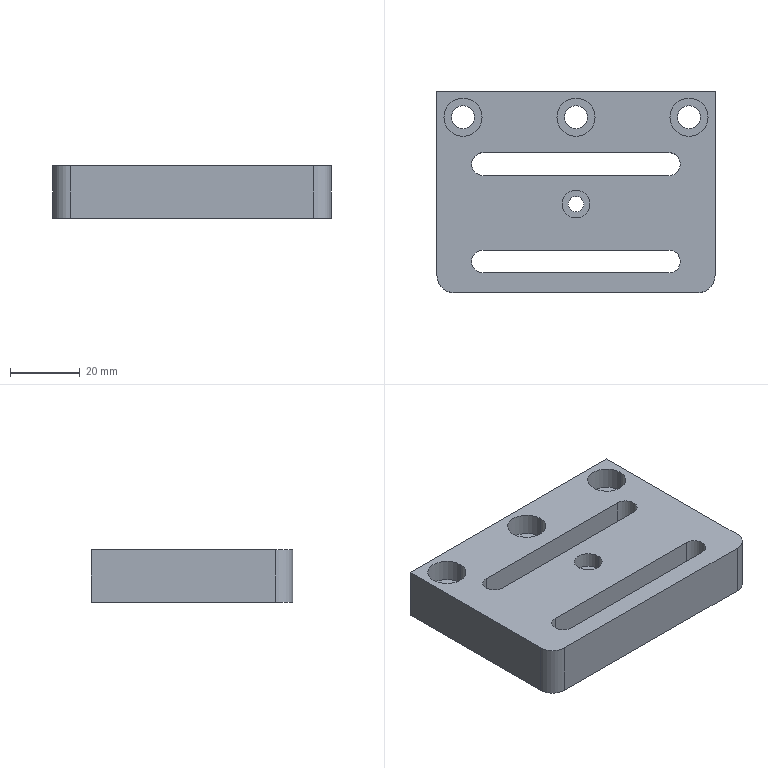Part | SolidWorks | features HoleWzd 3, Extrusion 1, Fillet 1 | 1 solid | 50 faces | box 80 x 58 x 15 mm | volume 50956 mm3 | cylinder 30 | plane 20 | commonest cylinder face diameters 6.6 x12 11 x12 4.5 x2 8 x2 10 x2
STEP:
#1=CARTESIAN_POINT('',(-38.,21.5,8.6));
#2=VERTEX_POINT('',#1);
#3=CARTESIAN_POINT('',(-27.,21.5,8.6));
#4=VERTEX_POINT('',#3);
#5=CARTESIAN_POINT('',(-32.5,21.5,8.6));
#6=DIRECTION('',(0.,0.,1.));
#7=DIRECTION('',(1.,0.,0.));
#8=AXIS2_PLACEMENT_3D('',#5,#6,#7);
#9=CIRCLE('',#8,5.5);
#10=EDGE_CURVE('',#2,#4,#9,.T.);
#11=ORIENTED_EDGE('',*,*,#10,.F.);
#12=CARTESIAN_POINT('',(-38.,21.5,15.));
#13=VERTEX_POINT('',#12);
#14=CARTESIAN_POINT('',(-38.,21.5,15.));
#15=DIRECTION('',(0.,0.,1.));
#16=VECTOR('',#15,1000.);
#17=LINE('',#14,#16);
#18=EDGE_CURVE('',#2,#13,#17,.T.);
#19=ORIENTED_EDGE('',*,*,#18,.T.);
#20=CARTESIAN_POINT('',(-27.,21.5,15.));
#21=VERTEX_POINT('',#20);
#22=CARTESIAN_POINT('',(-32.5,21.5,15.));
#23=DIRECTION('',(0.,0.,1.));
#24=DIRECTION('',(1.,0.,0.));
#25=AXIS2_PLACEMENT_3D('',#22,#23,#24);
#26=CIRCLE('',#25,5.5);
#27=EDGE_CURVE('',#13,#21,#26,.T.);
#28=ORIENTED_EDGE('',*,*,#27,.T.);
#29=CARTESIAN_POINT('',(-27.,21.5,15.));
#30=DIRECTION('',(0.,0.,1.));
#31=VECTOR('',#30,1000.);
#32=LINE('',#29,#31);
#33=EDGE_CURVE('',#4,#21,#32,.T.);
#34=ORIENTED_EDGE('',*,*,#33,.F.);
#35=EDGE_LOOP('',(#11,#19,#28,#34));
#36=FACE_OUTER_BOUND('',#35,.T.);
#37=CARTESIAN_POINT('',(-32.5,21.5,15.));
#38=DIRECTION('',(0.,0.,1.));
#39=DIRECTION('',(1.,0.,0.));
#40=AXIS2_PLACEMENT_3D('',#37,#38,#39);
#41=CYLINDRICAL_SURFACE('',#40,5.5);
#42=ADVANCED_FACE('',(#36),#41,.F.);
#43=CARTESIAN_POINT('',(-35.8,21.5,0.));
#44=VERTEX_POINT('',#43);
#45=CARTESIAN_POINT('',(-29.2,21.5,0.));
#46=VERTEX_POINT('',#45);
#47=CARTESIAN_POINT('',(-32.5,21.5,0.));
#48=DIRECTION('',(0.,0.,1.));
#49=DIRECTION('',(1.,0.,0.));
#50=AXIS2_PLACEMENT_3D('',#47,#48,#49);
#51=CIRCLE('',#50,3.3);
#52=EDGE_CURVE('',#44,#46,#51,.T.);
#53=ORIENTED_EDGE('',*,*,#52,.F.);
#54=CARTESIAN_POINT('',(-35.8,21.5,8.6));
#55=VERTEX_POINT('',#54);
#56=CARTESIAN_POINT('',(-35.8,21.5,15.));
#57=DIRECTION('',(0.,0.,1.));
#58=VECTOR('',#57,1000.);
#59=LINE('',#56,#58);
#60=EDGE_CURVE('',#44,#55,#59,.T.);
#61=ORIENTED_EDGE('',*,*,#60,.T.);
#62=CARTESIAN_POINT('',(-29.2,21.5,8.6));
#63=VERTEX_POINT('',#62);
#64=CARTESIAN_POINT('',(-32.5,21.5,8.6));
#65=DIRECTION('',(0.,0.,1.));
#66=DIRECTION('',(1.,0.,0.));
#67=AXIS2_PLACEMENT_3D('',#64,#65,#66);
#68=CIRCLE('',#67,3.3);
#69=EDGE_CURVE('',#55,#63,#68,.T.);
#70=ORIENTED_EDGE('',*,*,#69,.T.);
#71=CARTESIAN_POINT('',(-29.2,21.5,15.));
#72=DIRECTION('',(0.,0.,1.));
#73=VECTOR('',#72,1000.);
#74=LINE('',#71,#73);
#75=EDGE_CURVE('',#46,#63,#74,.T.);
#76=ORIENTED_EDGE('',*,*,#75,.F.);
#77=EDGE_LOOP('',(#53,#61,#70,#76));
#78=FACE_OUTER_BOUND('',#77,.T.);
#79=CARTESIAN_POINT('',(-32.5,21.5,15.));
#80=DIRECTION('',(0.,0.,1.));
#81=DIRECTION('',(1.,0.,0.));
#82=AXIS2_PLACEMENT_3D('',#79,#80,#81);
#83=CYLINDRICAL_SURFACE('',#82,3.3);
#84=ADVANCED_FACE('',(#78),#83,.F.);
#85=CARTESIAN_POINT('',(-5.5,21.5,8.6));
#86=VERTEX_POINT('',#85);
#87=CARTESIAN_POINT('',(5.5,21.5,8.6));
#88=VERTEX_POINT('',#87);
#89=CARTESIAN_POINT('',(0.,21.5,8.6));
#90=DIRECTION('',(0.,0.,1.));
#91=DIRECTION('',(1.,0.,0.));
#92=AXIS2_PLACEMENT_3D('',#89,#90,#91);
#93=CIRCLE('',#92,5.5);
#94=EDGE_CURVE('',#86,#88,#93,.T.);
#95=ORIENTED_EDGE('',*,*,#94,.F.);
#96=CARTESIAN_POINT('',(-5.5,21.5,15.));
#97=VERTEX_POINT('',#96);
#98=CARTESIAN_POINT('',(-5.5,21.5,15.));
#99=DIRECTION('',(0.,0.,1.));
#100=VECTOR('',#99,1000.);
#101=LINE('',#98,#100);
#102=EDGE_CURVE('',#86,#97,#101,.T.);
#103=ORIENTED_EDGE('',*,*,#102,.T.);
#104=CARTESIAN_POINT('',(5.5,21.5,15.));
#105=VERTEX_POINT('',#104);
#106=CARTESIAN_POINT('',(0.,21.5,15.));
#107=DIRECTION('',(0.,0.,1.));
#108=DIRECTION('',(1.,0.,0.));
#109=AXIS2_PLACEMENT_3D('',#106,#107,#108);
#110=CIRCLE('',#109,5.5);
#111=EDGE_CURVE('',#97,#105,#110,.T.);
#112=ORIENTED_EDGE('',*,*,#111,.T.);
#113=CARTESIAN_POINT('',(5.5,21.5,15.));
#114=DIRECTION('',(0.,0.,1.));
#115=VECTOR('',#114,1000.);
#116=LINE('',#113,#115);
#117=EDGE_CURVE('',#88,#105,#116,.T.);
#118=ORIENTED_EDGE('',*,*,#117,.F.);
#119=EDGE_LOOP('',(#95,#103,#112,#118));
#120=FACE_OUTER_BOUND('',#119,.T.);
#121=CARTESIAN_POINT('',(0.,21.5,15.));
#122=DIRECTION('',(0.,0.,1.));
#123=DIRECTION('',(1.,0.,0.));
#124=AXIS2_PLACEMENT_3D('',#121,#122,#123);
#125=CYLINDRICAL_SURFACE('',#124,5.5);
#126=ADVANCED_FACE('',(#120),#125,.F.);
#127=CARTESIAN_POINT('',(-3.3,21.5,0.));
#128=VERTEX_POINT('',#127);
#129=CARTESIAN_POINT('',(3.3,21.5,0.));
#130=VERTEX_POINT('',#129);
#131=CARTESIAN_POINT('',(0.,21.5,0.));
#132=DIRECTION('',(0.,0.,1.));
#133=DIRECTION('',(1.,0.,0.));
#134=AXIS2_PLACEMENT_3D('',#131,#132,#133);
#135=CIRCLE('',#134,3.3);
#136=EDGE_CURVE('',#128,#130,#135,.T.);
#137=ORIENTED_EDGE('',*,*,#136,.F.);
#138=CARTESIAN_POINT('',(-3.3,21.5,8.6));
#139=VERTEX_POINT('',#138);
#140=CARTESIAN_POINT('',(-3.3,21.5,15.));
#141=DIRECTION('',(0.,0.,1.));
#142=VECTOR('',#141,1000.);
#143=LINE('',#140,#142);
#144=EDGE_CURVE('',#128,#139,#143,.T.);
#145=ORIENTED_EDGE('',*,*,#144,.T.);
#146=CARTESIAN_POINT('',(3.3,21.5,8.6));
#147=VERTEX_POINT('',#146);
#148=CARTESIAN_POINT('',(0.,21.5,8.6));
#149=DIRECTION('',(0.,0.,1.));
#150=DIRECTION('',(1.,0.,0.));
#151=AXIS2_PLACEMENT_3D('',#148,#149,#150);
#152=CIRCLE('',#151,3.3);
#153=EDGE_CURVE('',#139,#147,#152,.T.);
#154=ORIENTED_EDGE('',*,*,#153,.T.);
#155=CARTESIAN_POINT('',(3.3,21.5,15.));
#156=DIRECTION('',(0.,0.,1.));
#157=VECTOR('',#156,1000.);
#158=LINE('',#155,#157);
#159=EDGE_CURVE('',#130,#147,#158,.T.);
#160=ORIENTED_EDGE('',*,*,#159,.F.);
#161=EDGE_LOOP('',(#137,#145,#154,#160));
#162=FACE_OUTER_BOUND('',#161,.T.);
#163=CARTESIAN_POINT('',(0.,21.5,15.));
#164=DIRECTION('',(0.,0.,1.));
#165=DIRECTION('',(1.,0.,0.));
#166=AXIS2_PLACEMENT_3D('',#163,#164,#165);
#167=CYLINDRICAL_SURFACE('',#166,3.3);
#168=ADVANCED_FACE('',(#162),#167,.F.);
#169=CARTESIAN_POINT('',(27.,21.5,8.6));
#170=VERTEX_POINT('',#169);
#171=CARTESIAN_POINT('',(38.,21.5,8.6));
#172=VERTEX_POINT('',#171);
#173=CARTESIAN_POINT('',(32.5,21.5,8.6));
#174=DIRECTION('',(0.,0.,1.));
#175=DIRECTION('',(1.,0.,0.));
#176=AXIS2_PLACEMENT_3D('',#173,#174,#175);
#177=CIRCLE('',#176,5.5);
#178=EDGE_CURVE('',#170,#172,#177,.T.);
#179=ORIENTED_EDGE('',*,*,#178,.F.);
#180=CARTESIAN_POINT('',(27.,21.5,15.));
#181=VERTEX_POINT('',#180);
#182=CARTESIAN_POINT('',(27.,21.5,15.));
#183=DIRECTION('',(0.,0.,1.));
#184=VECTOR('',#183,1000.);
#185=LINE('',#182,#184);
#186=EDGE_CURVE('',#170,#181,#185,.T.);
#187=ORIENTED_EDGE('',*,*,#186,.T.);
#188=CARTESIAN_POINT('',(38.,21.5,15.));
#189=VERTEX_POINT('',#188);
#190=CARTESIAN_POINT('',(32.5,21.5,15.));
#191=DIRECTION('',(0.,0.,1.));
#192=DIRECTION('',(1.,0.,0.));
#193=AXIS2_PLACEMENT_3D('',#190,#191,#192);
#194=CIRCLE('',#193,5.5);
#195=EDGE_CURVE('',#181,#189,#194,.T.);
#196=ORIENTED_EDGE('',*,*,#195,.T.);
#197=CARTESIAN_POINT('',(38.,21.5,15.));
#198=DIRECTION('',(0.,0.,1.));
#199=VECTOR('',#198,1000.);
#200=LINE('',#197,#199);
#201=EDGE_CURVE('',#172,#189,#200,.T.);
#202=ORIENTED_EDGE('',*,*,#201,.F.);
#203=EDGE_LOOP('',(#179,#187,#196,#202));
#204=FACE_OUTER_BOUND('',#203,.T.);
#205=CARTESIAN_POINT('',(32.5,21.5,15.));
#206=DIRECTION('',(0.,0.,1.));
#207=DIRECTION('',(1.,0.,0.));
#208=AXIS2_PLACEMENT_3D('',#205,#206,#207);
#209=CYLINDRICAL_SURFACE('',#208,5.5);
#210=ADVANCED_FACE('',(#204),#209,.F.);
#211=CARTESIAN_POINT('',(29.2,21.5,0.));
#212=VERTEX_POINT('',#211);
#213=CARTESIAN_POINT('',(35.8,21.5,0.));
#214=VERTEX_POINT('',#213);
#215=CARTESIAN_POINT('',(32.5,21.5,0.));
#216=DIRECTION('',(0.,0.,1.));
#217=DIRECTION('',(1.,0.,0.));
#218=AXIS2_PLACEMENT_3D('',#215,#216,#217);
#219=CIRCLE('',#218,3.3);
#220=EDGE_CURVE('',#212,#214,#219,.T.);
#221=ORIENTED_EDGE('',*,*,#220,.F.);
#222=CARTESIAN_POINT('',(29.2,21.5,8.6));
#223=VERTEX_POINT('',#222);
#224=CARTESIAN_POINT('',(29.2,21.5,15.));
#225=DIRECTION('',(0.,0.,1.));
#226=VECTOR('',#225,1000.);
#227=LINE('',#224,#226);
#228=EDGE_CURVE('',#212,#223,#227,.T.);
#229=ORIENTED_EDGE('',*,*,#228,.T.);
#230=CARTESIAN_POINT('',(35.8,21.5,8.6));
#231=VERTEX_POINT('',#230);
#232=CARTESIAN_POINT('',(32.5,21.5,8.6));
#233=DIRECTION('',(0.,0.,1.));
#234=DIRECTION('',(1.,0.,0.));
#235=AXIS2_PLACEMENT_3D('',#232,#233,#234);
#236=CIRCLE('',#235,3.3);
#237=EDGE_CURVE('',#223,#231,#236,.T.);
#238=ORIENTED_EDGE('',*,*,#237,.T.);
#239=CARTESIAN_POINT('',(35.8,21.5,15.));
#240=DIRECTION('',(0.,0.,1.));
#241=VECTOR('',#240,1000.);
#242=LINE('',#239,#241);
#243=EDGE_CURVE('',#214,#231,#242,.T.);
#244=ORIENTED_EDGE('',*,*,#243,.F.);
#245=EDGE_LOOP('',(#221,#229,#238,#244));
#246=FACE_OUTER_BOUND('',#245,.T.);
#247=CARTESIAN_POINT('',(32.5,21.5,15.));
#248=DIRECTION('',(0.,0.,1.));
#249=DIRECTION('',(1.,0.,0.));
#250=AXIS2_PLACEMENT_3D('',#247,#248,#249);
#251=CYLINDRICAL_SURFACE('',#250,3.3);
#252=ADVANCED_FACE('',(#246),#251,.F.);
#253=CARTESIAN_POINT('',(-4.,-3.5,10.6));
#254=VERTEX_POINT('',#253);
#255=CARTESIAN_POINT('',(4.,-3.5,10.6));
#256=VERTEX_POINT('',#255);
#257=CARTESIAN_POINT('',(0.,-3.5,10.6));
#258=DIRECTION('',(0.,0.,1.));
#259=DIRECTION('',(1.,0.,0.));
#260=AXIS2_PLACEMENT_3D('',#257,#258,#259);
#261=CIRCLE('',#260,4.);
#262=EDGE_CURVE('',#254,#256,#261,.T.);
#263=ORIENTED_EDGE('',*,*,#262,.F.);
#264=CARTESIAN_POINT('',(-4.,-3.5,15.));
#265=VERTEX_POINT('',#264);
#266=CARTESIAN_POINT('',(-4.,-3.5,15.));
#267=DIRECTION('',(0.,0.,1.));
#268=VECTOR('',#267,1000.);
#269=LINE('',#266,#268);
#270=EDGE_CURVE('',#254,#265,#269,.T.);
#271=ORIENTED_EDGE('',*,*,#270,.T.);
#272=CARTESIAN_POINT('',(4.,-3.5,15.));
#273=VERTEX_POINT('',#272);
#274=CARTESIAN_POINT('',(0.,-3.5,15.));
#275=DIRECTION('',(0.,0.,1.));
#276=DIRECTION('',(1.,0.,0.));
#277=AXIS2_PLACEMENT_3D('',#274,#275,#276);
#278=CIRCLE('',#277,4.);
#279=EDGE_CURVE('',#265,#273,#278,.T.);
#280=ORIENTED_EDGE('',*,*,#279,.T.);
#281=CARTESIAN_POINT('',(4.,-3.5,15.));
#282=DIRECTION('',(0.,0.,1.));
#283=VECTOR('',#282,1000.);
#284=LINE('',#281,#283);
#285=EDGE_CURVE('',#256,#273,#284,.T.);
#286=ORIENTED_EDGE('',*,*,#285,.F.);
#287=EDGE_LOOP('',(#263,#271,#280,#286));
#288=FACE_OUTER_BOUND('',#287,.T.);
#289=CARTESIAN_POINT('',(0.,-3.5,15.));
#290=DIRECTION('',(0.,0.,1.));
#291=DIRECTION('',(1.,0.,0.));
#292=AXIS2_PLACEMENT_3D('',#289,#290,#291);
#293=CYLINDRICAL_SURFACE('',#292,4.);
#294=ADVANCED_FACE('',(#288),#293,.F.);
#295=CARTESIAN_POINT('',(-2.25,-3.5,0.));
#296=VERTEX_POINT('',#295);
#297=CARTESIAN_POINT('',(2.25,-3.5,0.));
#298=VERTEX_POINT('',#297);
#299=CARTESIAN_POINT('',(0.,-3.5,0.));
#300=DIRECTION('',(0.,0.,1.));
#301=DIRECTION('',(1.,0.,0.));
#302=AXIS2_PLACEMENT_3D('',#299,#300,#301);
#303=CIRCLE('',#302,2.25);
#304=EDGE_CURVE('',#296,#298,#303,.T.);
#305=ORIENTED_EDGE('',*,*,#304,.F.);
#306=CARTESIAN_POINT('',(-2.25,-3.5,10.6));
#307=VERTEX_POINT('',#306);
#308=CARTESIAN_POINT('',(-2.25,-3.5,15.));
#309=DIRECTION('',(0.,0.,1.));
#310=VECTOR('',#309,1000.);
#311=LINE('',#308,#310);
#312=EDGE_CURVE('',#296,#307,#311,.T.);
#313=ORIENTED_EDGE('',*,*,#312,.T.);
#314=CARTESIAN_POINT('',(2.25,-3.5,10.6));
#315=VERTEX_POINT('',#314);
#316=CARTESIAN_POINT('',(0.,-3.5,10.6));
#317=DIRECTION('',(0.,0.,1.));
#318=DIRECTION('',(1.,0.,0.));
#319=AXIS2_PLACEMENT_3D('',#316,#317,#318);
#320=CIRCLE('',#319,2.25);
#321=EDGE_CURVE('',#307,#315,#320,.T.);
#322=ORIENTED_EDGE('',*,*,#321,.T.);
#323=CARTESIAN_POINT('',(2.25,-3.5,15.));
#324=DIRECTION('',(0.,0.,1.));
#325=VECTOR('',#324,1000.);
#326=LINE('',#323,#325);
#327=EDGE_CURVE('',#298,#315,#326,.T.);
#328=ORIENTED_EDGE('',*,*,#327,.F.);
#329=EDGE_LOOP('',(#305,#313,#322,#328));
#330=FACE_OUTER_BOUND('',#329,.T.);
#331=CARTESIAN_POINT('',(0.,-3.5,15.));
#332=DIRECTION('',(0.,0.,1.));
#333=DIRECTION('',(1.,0.,0.));
#334=AXIS2_PLACEMENT_3D('',#331,#332,#333);
#335=CYLINDRICAL_SURFACE('',#334,2.25);
#336=ADVANCED_FACE('',(#330),#335,.F.);
#337=CARTESIAN_POINT('',(-32.2,-20.,6.4));
#338=VERTEX_POINT('',#337);
#339=CARTESIAN_POINT('',(-26.7,-14.5,6.4));
#340=VERTEX_POINT('',#339);
#341=CARTESIAN_POINT('',(-26.7,-20.,6.4));
#342=DIRECTION('',(0.,0.,-1.));
#343=DIRECTION('',(-1.,0.,0.));
#344=AXIS2_PLACEMENT_3D('',#341,#342,#343);
#345=CIRCLE('',#344,5.5);
#346=EDGE_CURVE('',#338,#340,#345,.T.);
#347=ORIENTED_EDGE('',*,*,#346,.F.);
#348=CARTESIAN_POINT('',(-32.2,-20.,0.));
#349=VERTEX_POINT('',#348);
#350=CARTESIAN_POINT('',(-32.2,-20.,0.));
#351=DIRECTION('',(0.,0.,-1.));
#352=VECTOR('',#351,1000.);
#353=LINE('',#350,#352);
#354=EDGE_CURVE('',#338,#349,#353,.T.);
#355=ORIENTED_EDGE('',*,*,#354,.T.);
#356=CARTESIAN_POINT('',(-26.7,-14.5,0.));
#357=VERTEX_POINT('',#356);
#358=CARTESIAN_POINT('',(-26.7,-20.,0.));
#359=DIRECTION('',(0.,0.,-1.));
#360=DIRECTION('',(-1.,0.,0.));
#361=AXIS2_PLACEMENT_3D('',#358,#359,#360);
#362=CIRCLE('',#361,5.5);
#363=EDGE_CURVE('',#349,#357,#362,.T.);
#364=ORIENTED_EDGE('',*,*,#363,.T.);
#365=CARTESIAN_POINT('',(-26.7,-14.5,0.));
#366=DIRECTION('',(0.,0.,-1.));
#367=VECTOR('',#366,1000.);
#368=LINE('',#365,#367);
#369=EDGE_CURVE('',#340,#357,#368,.T.);
#370=ORIENTED_EDGE('',*,*,#369,.F.);
#371=EDGE_LOOP('',(#347,#355,#364,#370));
#372=FACE_OUTER_BOUND('',#371,.T.);
#373=CARTESIAN_POINT('',(-26.7,-20.,0.));
#374=DIRECTION('',(0.,0.,-1.));
#375=DIRECTION('',(-1.,0.,0.));
#376=AXIS2_PLACEMENT_3D('',#373,#374,#375);
#377=CYLINDRICAL_SURFACE('',#376,5.5);
#378=ADVANCED_FACE('',(#372),#377,.F.);
#379=CARTESIAN_POINT('',(-30.,-20.,15.));
#380=VERTEX_POINT('',#379);
#381=CARTESIAN_POINT('',(-26.7,-16.7,15.));
#382=VERTEX_POINT('',#381);
#383=CARTESIAN_POINT('',(-26.7,-20.,15.));
#384=DIRECTION('',(0.,0.,-1.));
#385=DIRECTION('',(-1.,0.,0.));
#386=AXIS2_PLACEMENT_3D('',#383,#384,#385);
#387=CIRCLE('',#386,3.3);
#388=EDGE_CURVE('',#380,#382,#387,.T.);
#389=ORIENTED_EDGE('',*,*,#388,.F.);
#390=CARTESIAN_POINT('',(-30.,-20.,6.4));
#391=VERTEX_POINT('',#390);
#392=CARTESIAN_POINT('',(-30.,-20.,0.));
#393=DIRECTION('',(0.,0.,-1.));
#394=VECTOR('',#393,1000.);
#395=LINE('',#392,#394);
#396=EDGE_CURVE('',#380,#391,#395,.T.);
#397=ORIENTED_EDGE('',*,*,#396,.T.);
#398=CARTESIAN_POINT('',(-26.7,-16.7,6.4));
#399=VERTEX_POINT('',#398);
#400=CARTESIAN_POINT('',(-26.7,-20.,6.4));
#401=DIRECTION('',(0.,0.,-1.));
#402=DIRECTION('',(-1.,0.,0.));
#403=AXIS2_PLACEMENT_3D('',#400,#401,#402);
#404=CIRCLE('',#403,3.3);
#405=EDGE_CURVE('',#391,#399,#404,.T.);
#406=ORIENTED_EDGE('',*,*,#405,.T.);
#407=CARTESIAN_POINT('',(-26.7,-16.7,0.));
#408=DIRECTION('',(0.,0.,-1.));
#409=VECTOR('',#408,1000.);
#410=LINE('',#407,#409);
#411=EDGE_CURVE('',#382,#399,#410,.T.);
#412=ORIENTED_EDGE('',*,*,#411,.F.);
#413=EDGE_LOOP('',(#389,#397,#406,#412));
#414=FACE_OUTER_BOUND('',#413,.T.);
#415=CARTESIAN_POINT('',(-26.7,-20.,0.));
#416=DIRECTION('',(0.,0.,-1.));
#417=DIRECTION('',(-1.,0.,0.));
#418=AXIS2_PLACEMENT_3D('',#415,#416,#417);
#419=CYLINDRICAL_SURFACE('',#418,3.3);
#420=ADVANCED_FACE('',(#414),#419,.F.);
#421=CARTESIAN_POINT('',(-32.2,8.,6.4));
#422=VERTEX_POINT('',#421);
#423=CARTESIAN_POINT('',(-26.7,13.5,6.4));
#424=VERTEX_POINT('',#423);
#425=CARTESIAN_POINT('',(-26.7,8.,6.4));
#426=DIRECTION('',(0.,0.,-1.));
#427=DIRECTION('',(-1.,0.,0.));
#428=AXIS2_PLACEMENT_3D('',#425,#426,#427);
#429=CIRCLE('',#428,5.5);
#430=EDGE_CURVE('',#422,#424,#429,.T.);
#431=ORIENTED_EDGE('',*,*,#430,.F.);
#432=CARTESIAN_POINT('',(-32.2,8.,0.));
#433=VERTEX_POINT('',#432);
#434=CARTESIAN_POINT('',(-32.2,8.,0.));
#435=DIRECTION('',(0.,0.,-1.));
#436=VECTOR('',#435,1000.);
#437=LINE('',#434,#436);
#438=EDGE_CURVE('',#422,#433,#437,.T.);
#439=ORIENTED_EDGE('',*,*,#438,.T.);
#440=CARTESIAN_POINT('',(-26.7,13.5,0.));
#441=VERTEX_POINT('',#440);
#442=CARTESIAN_POINT('',(-26.7,8.,0.));
#443=DIRECTION('',(0.,0.,-1.));
#444=DIRECTION('',(-1.,0.,0.));
#445=AXIS2_PLACEMENT_3D('',#442,#443,#444);
#446=CIRCLE('',#445,5.5);
#447=EDGE_CURVE('',#433,#441,#446,.T.);
#448=ORIENTED_EDGE('',*,*,#447,.T.);
#449=CARTESIAN_POINT('',(-26.7,13.5,0.));
#450=DIRECTION('',(0.,0.,-1.));
#451=VECTOR('',#450,1000.);
#452=LINE('',#449,#451);
#453=EDGE_CURVE('',#424,#441,#452,.T.);
#454=ORIENTED_EDGE('',*,*,#453,.F.);
#455=EDGE_LOOP('',(#431,#439,#448,#454));
#456=FACE_OUTER_BOUND('',#455,.T.);
#457=CARTESIAN_POINT('',(-26.7,8.,0.));
#458=DIRECTION('',(0.,0.,-1.));
#459=DIRECTION('',(-1.,0.,0.));
#460=AXIS2_PLACEMENT_3D('',#457,#458,#459);
#461=CYLINDRICAL_SURFACE('',#460,5.5);
#462=ADVANCED_FACE('',(#456),#461,.F.);
#463=CARTESIAN_POINT('',(-30.,8.,15.));
#464=VERTEX_POINT('',#463);
#465=CARTESIAN_POINT('',(-26.7,11.3,15.));
#466=VERTEX_POINT('',#465);
#467=CARTESIAN_POINT('',(-26.7,8.,15.));
#468=DIRECTION('',(0.,0.,-1.));
#469=DIRECTION('',(-1.,0.,0.));
#470=AXIS2_PLACEMENT_3D('',#467,#468,#469);
#471=CIRCLE('',#470,3.3);
#472=EDGE_CURVE('',#464,#466,#471,.T.);
#473=ORIENTED_EDGE('',*,*,#472,.F.);
#474=CARTESIAN_POINT('',(-30.,8.,6.4));
#475=VERTEX_POINT('',#474);
#476=CARTESIAN_POINT('',(-30.,8.,0.));
#477=DIRECTION('',(0.,0.,-1.));
#478=VECTOR('',#477,1000.);
#479=LINE('',#476,#478);
#480=EDGE_CURVE('',#464,#475,#479,.T.);
#481=ORIENTED_EDGE('',*,*,#480,.T.);
#482=CARTESIAN_POINT('',(-26.7,11.3,6.4));
#483=VERTEX_POINT('',#482);
#484=CARTESIAN_POINT('',(-26.7,8.,6.4));
#485=DIRECTION('',(0.,0.,-1.));
#486=DIRECTION('',(-1.,0.,0.));
#487=AXIS2_PLACEMENT_3D('',#484,#485,#486);
#488=CIRCLE('',#487,3.3);
#489=EDGE_CURVE('',#475,#483,#488,.T.);
#490=ORIENTED_EDGE('',*,*,#489,.T.);
#491=CARTESIAN_POINT('',(-26.7,11.3,0.));
#492=DIRECTION('',(0.,0.,-1.));
#493=VECTOR('',#492,1000.);
#494=LINE('',#491,#493);
#495=EDGE_CURVE('',#466,#483,#494,.T.);
#496=ORIENTED_EDGE('',*,*,#495,.F.);
#497=EDGE_LOOP('',(#473,#481,#490,#496));
#498=FACE_OUTER_BOUND('',#497,.T.);
#499=CARTESIAN_POINT('',(-26.7,8.,0.));
#500=DIRECTION('',(0.,0.,-1.));
#501=DIRECTION('',(-1.,0.,0.));
#502=AXIS2_PLACEMENT_3D('',#499,#500,#501);
#503=CYLINDRICAL_SURFACE('',#502,3.3);
#504=ADVANCED_FACE('',(#498),#503,.F.);
#505=CARTESIAN_POINT('',(40.,-24.,15.));
#506=VERTEX_POINT('',#505);
#507=CARTESIAN_POINT('',(40.,29.,15.));
#508=VERTEX_POINT('',#507);
#509=CARTESIAN_POINT('',(40.,29.,15.));
#510=DIRECTION('',(0.,1.,0.));
#511=VECTOR('',#510,1000.);
#512=LINE('',#509,#511);
#513=EDGE_CURVE('',#506,#508,#512,.T.);
#514=ORIENTED_EDGE('',*,*,#513,.F.);
#515=CARTESIAN_POINT('',(40.,-24.,0.));
#516=VERTEX_POINT('',#515);
#517=CARTESIAN_POINT('',(40.,-24.,15.));
#518=DIRECTION('',(0.,0.,-1.));
#519=VECTOR('',#518,1000.);
#520=LINE('',#517,#519);
#521=EDGE_CURVE('',#506,#516,#520,.T.);
#522=ORIENTED_EDGE('',*,*,#521,.T.);
#523=CARTESIAN_POINT('',(40.,29.,0.));
#524=VERTEX_POINT('',#523);
#525=CARTESIAN_POINT('',(40.,29.,0.));
#526=DIRECTION('',(0.,1.,0.));
#527=VECTOR('',#526,1000.);
#528=LINE('',#525,#527);
#529=EDGE_CURVE('',#516,#524,#528,.T.);
#530=ORIENTED_EDGE('',*,*,#529,.T.);
#531=CARTESIAN_POINT('',(40.,29.,15.));
#532=DIRECTION('',(0.,0.,-1.));
#533=VECTOR('',#532,1000.);
#534=LINE('',#531,#533);
#535=EDGE_CURVE('',#508,#524,#534,.T.);
#536=ORIENTED_EDGE('',*,*,#535,.F.);
#537=EDGE_LOOP('',(#514,#522,#530,#536));
#538=FACE_OUTER_BOUND('',#537,.T.);
#539=CARTESIAN_POINT('',(40.,29.,15.));
#540=DIRECTION('',(-1.,0.,0.));
#541=DIRECTION('',(0.,-1.,0.));
#542=AXIS2_PLACEMENT_3D('',#539,#540,#541);
#543=PLANE('',#542);
#544=ADVANCED_FACE('',(#538),#543,.F.);
#545=CARTESIAN_POINT('',(-40.,29.,0.));
#546=VERTEX_POINT('',#545);
#547=CARTESIAN_POINT('',(-40.,29.,0.));
#548=DIRECTION('',(-1.,0.,0.));
#549=VECTOR('',#548,1000.);
#550=LINE('',#547,#549);
#551=EDGE_CURVE('',#524,#546,#550,.T.);
#552=ORIENTED_EDGE('',*,*,#551,.T.);
#553=CARTESIAN_POINT('',(-40.,29.,15.));
#554=VERTEX_POINT('',#553);
#555=CARTESIAN_POINT('',(-40.,29.,15.));
#556=DIRECTION('',(0.,0.,-1.));
#557=VECTOR('',#556,1000.);
#558=LINE('',#555,#557);
#559=EDGE_CURVE('',#554,#546,#558,.T.);
#560=ORIENTED_EDGE('',*,*,#559,.F.);
#561=CARTESIAN_POINT('',(-40.,29.,15.));
#562=DIRECTION('',(-1.,0.,0.));
#563=VECTOR('',#562,1000.);
#564=LINE('',#561,#563);
#565=EDGE_CURVE('',#508,#554,#564,.T.);
#566=ORIENTED_EDGE('',*,*,#565,.F.);
#567=ORIENTED_EDGE('',*,*,#535,.T.);
#568=EDGE_LOOP('',(#552,#560,#566,#567));
#569=FACE_OUTER_BOUND('',#568,.T.);
#570=CARTESIAN_POINT('',(-40.,29.,15.));
#571=DIRECTION('',(0.,-1.,0.));
#572=DIRECTION('',(1.,0.,0.));
#573=AXIS2_PLACEMENT_3D('',#570,#571,#572);
#574=PLANE('',#573);
#575=ADVANCED_FACE('',(#569),#574,.F.);
#576=CARTESIAN_POINT('',(-40.,-24.,0.));
#577=VERTEX_POINT('',#576);
#578=CARTESIAN_POINT('',(-40.,29.,0.));
#579=DIRECTION('',(0.,-1.,0.));
#580=VECTOR('',#579,1000.);
#581=LINE('',#578,#580);
#582=EDGE_CURVE('',#546,#577,#581,.T.);
#583=ORIENTED_EDGE('',*,*,#582,.T.);
#584=CARTESIAN_POINT('',(-40.,-24.,15.));
#585=VERTEX_POINT('',#584);
#586=CARTESIAN_POINT('',(-40.,-24.,15.));
#587=DIRECTION('',(0.,0.,1.));
#588=VECTOR('',#587,1000.);
#589=LINE('',#586,#588);
#590=EDGE_CURVE('',#577,#585,#589,.T.);
#591=ORIENTED_EDGE('',*,*,#590,.T.);
#592=CARTESIAN_POINT('',(-40.,29.,15.));
#593=DIRECTION('',(0.,-1.,0.));
#594=VECTOR('',#593,1000.);
#595=LINE('',#592,#594);
#596=EDGE_CURVE('',#554,#585,#595,.T.);
#597=ORIENTED_EDGE('',*,*,#596,.F.);
#598=ORIENTED_EDGE('',*,*,#559,.T.);
#599=EDGE_LOOP('',(#583,#591,#597,#598));
#600=FACE_OUTER_BOUND('',#599,.T.);
#601=CARTESIAN_POINT('',(-40.,29.,15.));
#602=DIRECTION('',(1.,0.,0.));
#603=DIRECTION('',(0.,1.,0.));
#604=AXIS2_PLACEMENT_3D('',#601,#602,#603);
#605=PLANE('',#604);
#606=ADVANCED_FACE('',(#600),#605,.F.);
#607=CARTESIAN_POINT('',(-35.,-29.,0.));
#608=VERTEX_POINT('',#607);
#609=CARTESIAN_POINT('',(35.,-29.,0.));
#610=VERTEX_POINT('',#609);
#611=CARTESIAN_POINT('',(-40.,-29.,0.));
#612=DIRECTION('',(1.,0.,0.));
#613=VECTOR('',#612,1000.);
#614=LINE('',#611,#613);
#615=EDGE_CURVE('',#608,#610,#614,.T.);
#616=ORIENTED_EDGE('',*,*,#615,.T.);
#617=CARTESIAN_POINT('',(35.,-29.,15.));
#618=VERTEX_POINT('',#617);
#619=CARTESIAN_POINT('',(35.,-29.,15.));
#620=DIRECTION('',(0.,0.,1.));
#621=VECTOR('',#620,1000.);
#622=LINE('',#619,#621);
#623=EDGE_CURVE('',#610,#618,#622,.T.);
#624=ORIENTED_EDGE('',*,*,#623,.T.);
#625=CARTESIAN_POINT('',(-35.,-29.,15.));
#626=VERTEX_POINT('',#625);
#627=CARTESIAN_POINT('',(-40.,-29.,15.));
#628=DIRECTION('',(1.,0.,0.));
#629=VECTOR('',#628,1000.);
#630=LINE('',#627,#629);
#631=EDGE_CURVE('',#626,#618,#630,.T.);
#632=ORIENTED_EDGE('',*,*,#631,.F.);
#633=CARTESIAN_POINT('',(-35.,-29.,15.));
#634=DIRECTION('',(0.,0.,-1.));
#635=VECTOR('',#634,1000.);
#636=LINE('',#633,#635);
#637=EDGE_CURVE('',#626,#608,#636,.T.);
#638=ORIENTED_EDGE('',*,*,#637,.T.);
#639=EDGE_LOOP('',(#616,#624,#632,#638));
#640=FACE_OUTER_BOUND('',#639,.T.);
#641=CARTESIAN_POINT('',(-40.,-29.,15.));
#642=DIRECTION('',(0.,1.,0.));
#643=DIRECTION('',(0.,0.,1.));
#644=AXIS2_PLACEMENT_3D('',#641,#642,#643);
#645=PLANE('',#644);
#646=ADVANCED_FACE('',(#640),#645,.F.);
#647=CARTESIAN_POINT('',(-32.5,21.5,15.));
#648=DIRECTION('',(0.,0.,1.));
#649=DIRECTION('',(1.,0.,0.));
#650=AXIS2_PLACEMENT_3D('',#647,#648,#649);
#651=CIRCLE('',#650,5.5);
#652=EDGE_CURVE('',#21,#13,#651,.T.);
#653=ORIENTED_EDGE('',*,*,#652,.F.);
#654=ORIENTED_EDGE('',*,*,#27,.F.);
#655=EDGE_LOOP('',(#653,#654));
#656=FACE_BOUND('',#655,.T.);
#657=CARTESIAN_POINT('',(0.,21.5,15.));
#658=DIRECTION('',(0.,0.,1.));
#659=DIRECTION('',(1.,0.,0.));
#660=AXIS2_PLACEMENT_3D('',#657,#658,#659);
#661=CIRCLE('',#660,5.5);
#662=EDGE_CURVE('',#105,#97,#661,.T.);
#663=ORIENTED_EDGE('',*,*,#662,.F.);
#664=ORIENTED_EDGE('',*,*,#111,.F.);
#665=EDGE_LOOP('',(#663,#664));
#666=FACE_BOUND('',#665,.T.);
#667=CARTESIAN_POINT('',(32.5,21.5,15.));
#668=DIRECTION('',(0.,0.,1.));
#669=DIRECTION('',(1.,0.,0.));
#670=AXIS2_PLACEMENT_3D('',#667,#668,#669);
#671=CIRCLE('',#670,5.5);
#672=EDGE_CURVE('',#189,#181,#671,.T.);
#673=ORIENTED_EDGE('',*,*,#672,.F.);
#674=ORIENTED_EDGE('',*,*,#195,.F.);
#675=EDGE_LOOP('',(#673,#674));
#676=FACE_BOUND('',#675,.T.);
#677=CARTESIAN_POINT('',(0.,-3.5,15.));
#678=DIRECTION('',(0.,0.,1.));
#679=DIRECTION('',(1.,0.,0.));
#680=AXIS2_PLACEMENT_3D('',#677,#678,#679);
#681=CIRCLE('',#680,4.);
#682=EDGE_CURVE('',#273,#265,#681,.T.);
#683=ORIENTED_EDGE('',*,*,#682,.F.);
#684=ORIENTED_EDGE('',*,*,#279,.F.);
#685=EDGE_LOOP('',(#683,#684));
#686=FACE_BOUND('',#685,.T.);
#687=CARTESIAN_POINT('',(26.7,-16.7,15.));
#688=VERTEX_POINT('',#687);
#689=CARTESIAN_POINT('',(26.7,-23.3,15.));
#690=VERTEX_POINT('',#689);
#691=CARTESIAN_POINT('',(26.7,-20.,15.));
#692=DIRECTION('',(0.,0.,-1.));
#693=DIRECTION('',(-1.,0.,0.));
#694=AXIS2_PLACEMENT_3D('',#691,#692,#693);
#695=CIRCLE('',#694,3.3);
#696=EDGE_CURVE('',#688,#690,#695,.T.);
#697=ORIENTED_EDGE('',*,*,#696,.T.);
#698=CARTESIAN_POINT('',(-26.7,-23.3,15.));
#699=VERTEX_POINT('',#698);
#700=CARTESIAN_POINT('',(-26.7,-23.3,15.));
#701=DIRECTION('',(1.,0.,0.));
#702=VECTOR('',#701,1000.);
#703=LINE('',#700,#702);
#704=EDGE_CURVE('',#699,#690,#703,.T.);
#705=ORIENTED_EDGE('',*,*,#704,.F.);
#706=CARTESIAN_POINT('',(-26.7,-20.,15.));
#707=DIRECTION('',(0.,0.,-1.));
#708=DIRECTION('',(-1.,0.,0.));
#709=AXIS2_PLACEMENT_3D('',#706,#707,#708);
#710=CIRCLE('',#709,3.3);
#711=EDGE_CURVE('',#699,#380,#710,.T.);
#712=ORIENTED_EDGE('',*,*,#711,.T.);
#713=ORIENTED_EDGE('',*,*,#388,.T.);
#714=CARTESIAN_POINT('',(-26.7,-16.7,15.));
#715=DIRECTION('',(1.,0.,0.));
#716=VECTOR('',#715,1000.);
#717=LINE('',#714,#716);
#718=EDGE_CURVE('',#382,#688,#717,.T.);
#719=ORIENTED_EDGE('',*,*,#718,.T.);
#720=EDGE_LOOP('',(#697,#705,#712,#713,#719));
#721=FACE_BOUND('',#720,.T.);
#722=CARTESIAN_POINT('',(26.7,11.3,15.));
#723=VERTEX_POINT('',#722);
#724=CARTESIAN_POINT('',(26.7,4.7,15.));
#725=VERTEX_POINT('',#724);
#726=CARTESIAN_POINT('',(26.7,8.,15.));
#727=DIRECTION('',(0.,0.,-1.));
#728=DIRECTION('',(-1.,0.,0.));
#729=AXIS2_PLACEMENT_3D('',#726,#727,#728);
#730=CIRCLE('',#729,3.3);
#731=EDGE_CURVE('',#723,#725,#730,.T.);
#732=ORIENTED_EDGE('',*,*,#731,.T.);
#733=CARTESIAN_POINT('',(-26.7,4.7,15.));
#734=VERTEX_POINT('',#733);
#735=CARTESIAN_POINT('',(-26.7,4.7,15.));
#736=DIRECTION('',(1.,0.,0.));
#737=VECTOR('',#736,1000.);
#738=LINE('',#735,#737);
#739=EDGE_CURVE('',#734,#725,#738,.T.);
#740=ORIENTED_EDGE('',*,*,#739,.F.);
#741=CARTESIAN_POINT('',(-26.7,8.,15.));
#742=DIRECTION('',(0.,0.,-1.));
#743=DIRECTION('',(-1.,0.,0.));
#744=AXIS2_PLACEMENT_3D('',#741,#742,#743);
#745=CIRCLE('',#744,3.3);
#746=EDGE_CURVE('',#734,#464,#745,.T.);
#747=ORIENTED_EDGE('',*,*,#746,.T.);
#748=ORIENTED_EDGE('',*,*,#472,.T.);
#749=CARTESIAN_POINT('',(-26.7,11.3,15.));
#750=DIRECTION('',(1.,0.,0.));
#751=VECTOR('',#750,1000.);
#752=LINE('',#749,#751);
#753=EDGE_CURVE('',#466,#723,#752,.T.);
#754=ORIENTED_EDGE('',*,*,#753,.T.);
#755=EDGE_LOOP('',(#732,#740,#747,#748,#754));
#756=FACE_BOUND('',#755,.T.);
#757=ORIENTED_EDGE('',*,*,#631,.T.);
#758=CARTESIAN_POINT('',(35.,-24.,15.));
#759=DIRECTION('',(0.,0.,1.));
#760=DIRECTION('',(1.,0.,0.));
#761=AXIS2_PLACEMENT_3D('',#758,#759,#760);
#762=CIRCLE('',#761,5.);
#763=EDGE_CURVE('',#618,#506,#762,.T.);
#764=ORIENTED_EDGE('',*,*,#763,.T.);
#765=ORIENTED_EDGE('',*,*,#513,.T.);
#766=ORIENTED_EDGE('',*,*,#565,.T.);
#767=ORIENTED_EDGE('',*,*,#596,.T.);
#768=CARTESIAN_POINT('',(-35.,-24.,15.));
#769=DIRECTION('',(0.,0.,1.));
#770=DIRECTION('',(1.,0.,0.));
#771=AXIS2_PLACEMENT_3D('',#768,#769,#770);
#772=CIRCLE('',#771,5.);
#773=EDGE_CURVE('',#585,#626,#772,.T.);
#774=ORIENTED_EDGE('',*,*,#773,.T.);
#775=EDGE_LOOP('',(#757,#764,#765,#766,#767,#774));
#776=FACE_OUTER_BOUND('',#775,.T.);
#777=CARTESIAN_POINT('',(0.,0.,15.));
#778=DIRECTION('',(0.,0.,1.));
#779=DIRECTION('',(1.,0.,0.));
#780=AXIS2_PLACEMENT_3D('',#777,#778,#779);
#781=PLANE('',#780);
#782=ADVANCED_FACE('',(#656,#666,#676,#686,#721,#756,#776),#781,.T.);
#783=CARTESIAN_POINT('',(-32.5,21.5,0.));
#784=DIRECTION('',(0.,0.,1.));
#785=DIRECTION('',(1.,0.,0.));
#786=AXIS2_PLACEMENT_3D('',#783,#784,#785);
#787=CIRCLE('',#786,3.3);
#788=EDGE_CURVE('',#46,#44,#787,.T.);
#789=ORIENTED_EDGE('',*,*,#788,.T.);
#790=ORIENTED_EDGE('',*,*,#52,.T.);
#791=EDGE_LOOP('',(#789,#790));
#792=FACE_BOUND('',#791,.T.);
#793=CARTESIAN_POINT('',(0.,21.5,0.));
#794=DIRECTION('',(0.,0.,1.));
#795=DIRECTION('',(1.,0.,0.));
#796=AXIS2_PLACEMENT_3D('',#793,#794,#795);
#797=CIRCLE('',#796,3.3);
#798=EDGE_CURVE('',#130,#128,#797,.T.);
#799=ORIENTED_EDGE('',*,*,#798,.T.);
#800=ORIENTED_EDGE('',*,*,#136,.T.);
#801=EDGE_LOOP('',(#799,#800));
#802=FACE_BOUND('',#801,.T.);
#803=CARTESIAN_POINT('',(32.5,21.5,0.));
#804=DIRECTION('',(0.,0.,1.));
#805=DIRECTION('',(1.,0.,0.));
#806=AXIS2_PLACEMENT_3D('',#803,#804,#805);
#807=CIRCLE('',#806,3.3);
#808=EDGE_CURVE('',#214,#212,#807,.T.);
#809=ORIENTED_EDGE('',*,*,#808,.T.);
#810=ORIENTED_EDGE('',*,*,#220,.T.);
#811=EDGE_LOOP('',(#809,#810));
#812=FACE_BOUND('',#811,.T.);
#813=CARTESIAN_POINT('',(0.,-3.5,0.));
#814=DIRECTION('',(0.,0.,1.));
#815=DIRECTION('',(1.,0.,0.));
#816=AXIS2_PLACEMENT_3D('',#813,#814,#815);
#817=CIRCLE('',#816,2.25);
#818=EDGE_CURVE('',#298,#296,#817,.T.);
#819=ORIENTED_EDGE('',*,*,#818,.T.);
#820=ORIENTED_EDGE('',*,*,#304,.T.);
#821=EDGE_LOOP('',(#819,#820));
#822=FACE_BOUND('',#821,.T.);
#823=CARTESIAN_POINT('',(26.7,-14.5,0.));
#824=VERTEX_POINT('',#823);
#825=CARTESIAN_POINT('',(26.7,-25.5,0.));
#826=VERTEX_POINT('',#825);
#827=CARTESIAN_POINT('',(26.7,-20.,0.));
#828=DIRECTION('',(0.,0.,-1.));
#829=DIRECTION('',(-1.,0.,0.));
#830=AXIS2_PLACEMENT_3D('',#827,#828,#829);
#831=CIRCLE('',#830,5.5);
#832=EDGE_CURVE('',#824,#826,#831,.T.);
#833=ORIENTED_EDGE('',*,*,#832,.F.);
#834=CARTESIAN_POINT('',(-26.7,-14.5,0.));
#835=DIRECTION('',(1.,0.,0.));
#836=VECTOR('',#835,1000.);
#837=LINE('',#834,#836);
#838=EDGE_CURVE('',#357,#824,#837,.T.);
#839=ORIENTED_EDGE('',*,*,#838,.F.);
#840=ORIENTED_EDGE('',*,*,#363,.F.);
#841=CARTESIAN_POINT('',(-26.7,-25.5,0.));
#842=VERTEX_POINT('',#841);
#843=CARTESIAN_POINT('',(-26.7,-20.,0.));
#844=DIRECTION('',(0.,0.,-1.));
#845=DIRECTION('',(-1.,0.,0.));
#846=AXIS2_PLACEMENT_3D('',#843,#844,#845);
#847=CIRCLE('',#846,5.5);
#848=EDGE_CURVE('',#842,#349,#847,.T.);
#849=ORIENTED_EDGE('',*,*,#848,.F.);
#850=CARTESIAN_POINT('',(-26.7,-25.5,0.));
#851=DIRECTION('',(1.,0.,0.));
#852=VECTOR('',#851,1000.);
#853=LINE('',#850,#852);
#854=EDGE_CURVE('',#842,#826,#853,.T.);
#855=ORIENTED_EDGE('',*,*,#854,.T.);
#856=EDGE_LOOP('',(#833,#839,#840,#849,#855));
#857=FACE_BOUND('',#856,.T.);
#858=CARTESIAN_POINT('',(-26.7,2.5,0.));
#859=VERTEX_POINT('',#858);
#860=CARTESIAN_POINT('',(-26.7,8.,0.));
#861=DIRECTION('',(0.,0.,-1.));
#862=DIRECTION('',(-1.,0.,0.));
#863=AXIS2_PLACEMENT_3D('',#860,#861,#862);
#864=CIRCLE('',#863,5.5);
#865=EDGE_CURVE('',#859,#433,#864,.T.);
#866=ORIENTED_EDGE('',*,*,#865,.F.);
#867=CARTESIAN_POINT('',(26.7,2.5,0.));
#868=VERTEX_POINT('',#867);
#869=CARTESIAN_POINT('',(-26.7,2.5,0.));
#870=DIRECTION('',(1.,0.,0.));
#871=VECTOR('',#870,1000.);
#872=LINE('',#869,#871);
#873=EDGE_CURVE('',#859,#868,#872,.T.);
#874=ORIENTED_EDGE('',*,*,#873,.T.);
#875=CARTESIAN_POINT('',(26.7,13.5,0.));
#876=VERTEX_POINT('',#875);
#877=CARTESIAN_POINT('',(26.7,8.,0.));
#878=DIRECTION('',(0.,0.,-1.));
#879=DIRECTION('',(-1.,0.,0.));
#880=AXIS2_PLACEMENT_3D('',#877,#878,#879);
#881=CIRCLE('',#880,5.5);
#882=EDGE_CURVE('',#876,#868,#881,.T.);
#883=ORIENTED_EDGE('',*,*,#882,.F.);
#884=CARTESIAN_POINT('',(-26.7,13.5,0.));
#885=DIRECTION('',(1.,0.,0.));
#886=VECTOR('',#885,1000.);
#887=LINE('',#884,#886);
#888=EDGE_CURVE('',#441,#876,#887,.T.);
#889=ORIENTED_EDGE('',*,*,#888,.F.);
#890=ORIENTED_EDGE('',*,*,#447,.F.);
#891=EDGE_LOOP('',(#866,#874,#883,#889,#890));
#892=FACE_BOUND('',#891,.T.);
#893=ORIENTED_EDGE('',*,*,#529,.F.);
#894=CARTESIAN_POINT('',(35.,-24.,0.));
#895=DIRECTION('',(0.,0.,-1.));
#896=DIRECTION('',(1.,0.,0.));
#897=AXIS2_PLACEMENT_3D('',#894,#895,#896);
#898=CIRCLE('',#897,5.);
#899=EDGE_CURVE('',#516,#610,#898,.T.);
#900=ORIENTED_EDGE('',*,*,#899,.T.);
#901=ORIENTED_EDGE('',*,*,#615,.F.);
#902=CARTESIAN_POINT('',(-35.,-24.,0.));
#903=DIRECTION('',(0.,0.,-1.));
#904=DIRECTION('',(1.,0.,0.));
#905=AXIS2_PLACEMENT_3D('',#902,#903,#904);
#906=CIRCLE('',#905,5.);
#907=EDGE_CURVE('',#608,#577,#906,.T.);
#908=ORIENTED_EDGE('',*,*,#907,.T.);
#909=ORIENTED_EDGE('',*,*,#582,.F.);
#910=ORIENTED_EDGE('',*,*,#551,.F.);
#911=EDGE_LOOP('',(#893,#900,#901,#908,#909,#910));
#912=FACE_OUTER_BOUND('',#911,.T.);
#913=CARTESIAN_POINT('',(0.,0.,0.));
#914=DIRECTION('',(0.,0.,1.));
#915=DIRECTION('',(1.,0.,0.));
#916=AXIS2_PLACEMENT_3D('',#913,#914,#915);
#917=PLANE('',#916);
#918=ADVANCED_FACE('',(#792,#802,#812,#822,#857,#892,#912),#917,.F.);
#919=ORIENTED_EDGE('',*,*,#731,.F.);
#920=CARTESIAN_POINT('',(26.7,11.3,6.4));
#921=VERTEX_POINT('',#920);
#922=CARTESIAN_POINT('',(26.7,11.3,0.));
#923=DIRECTION('',(0.,0.,1.));
#924=VECTOR('',#923,1000.);
#925=LINE('',#922,#924);
#926=EDGE_CURVE('',#921,#723,#925,.T.);
#927=ORIENTED_EDGE('',*,*,#926,.F.);
#928=CARTESIAN_POINT('',(26.7,4.7,6.4));
#929=VERTEX_POINT('',#928);
#930=CARTESIAN_POINT('',(26.7,8.,6.4));
#931=DIRECTION('',(0.,0.,-1.));
#932=DIRECTION('',(-1.,0.,0.));
#933=AXIS2_PLACEMENT_3D('',#930,#931,#932);
#934=CIRCLE('',#933,3.3);
#935=EDGE_CURVE('',#921,#929,#934,.T.);
#936=ORIENTED_EDGE('',*,*,#935,.T.);
#937=CARTESIAN_POINT('',(26.7,4.7,0.));
#938=DIRECTION('',(0.,0.,-1.));
#939=VECTOR('',#938,1000.);
#940=LINE('',#937,#939);
#941=EDGE_CURVE('',#725,#929,#940,.T.);
#942=ORIENTED_EDGE('',*,*,#941,.F.);
#943=EDGE_LOOP('',(#919,#927,#936,#942));
#944=FACE_OUTER_BOUND('',#943,.T.);
#945=CARTESIAN_POINT('',(26.7,8.,0.));
#946=DIRECTION('',(0.,0.,-1.));
#947=DIRECTION('',(-1.,0.,0.));
#948=AXIS2_PLACEMENT_3D('',#945,#946,#947);
#949=CYLINDRICAL_SURFACE('',#948,3.3);
#950=ADVANCED_FACE('',(#944),#949,.F.);
#951=CARTESIAN_POINT('',(-26.7,11.3,6.4));
#952=DIRECTION('',(1.,0.,0.));
#953=VECTOR('',#952,1000.);
#954=LINE('',#951,#953);
#955=EDGE_CURVE('',#483,#921,#954,.T.);
#956=ORIENTED_EDGE('',*,*,#955,.F.);
#957=ORIENTED_EDGE('',*,*,#489,.F.);
#958=CARTESIAN_POINT('',(-26.7,4.7,6.4));
#959=VERTEX_POINT('',#958);
#960=CARTESIAN_POINT('',(-26.7,8.,6.4));
#961=DIRECTION('',(0.,0.,-1.));
#962=DIRECTION('',(-1.,0.,0.));
#963=AXIS2_PLACEMENT_3D('',#960,#961,#962);
#964=CIRCLE('',#963,3.3);
#965=EDGE_CURVE('',#959,#475,#964,.T.);
#966=ORIENTED_EDGE('',*,*,#965,.F.);
#967=CARTESIAN_POINT('',(-26.7,4.7,6.4));
#968=DIRECTION('',(1.,0.,0.));
#969=VECTOR('',#968,1000.);
#970=LINE('',#967,#969);
#971=EDGE_CURVE('',#959,#929,#970,.T.);
#972=ORIENTED_EDGE('',*,*,#971,.T.);
#973=ORIENTED_EDGE('',*,*,#935,.F.);
#974=EDGE_LOOP('',(#956,#957,#966,#972,#973));
#975=FACE_BOUND('',#974,.T.);
#976=CARTESIAN_POINT('',(26.7,13.5,6.4));
#977=VERTEX_POINT('',#976);
#978=CARTESIAN_POINT('',(26.7,2.5,6.4));
#979=VERTEX_POINT('',#978);
#980=CARTESIAN_POINT('',(26.7,8.,6.4));
#981=DIRECTION('',(0.,0.,-1.));
#982=DIRECTION('',(-1.,0.,0.));
#983=AXIS2_PLACEMENT_3D('',#980,#981,#982);
#984=CIRCLE('',#983,5.5);
#985=EDGE_CURVE('',#977,#979,#984,.T.);
#986=ORIENTED_EDGE('',*,*,#985,.T.);
#987=CARTESIAN_POINT('',(-26.7,2.5,6.4));
#988=VERTEX_POINT('',#987);
#989=CARTESIAN_POINT('',(-26.7,2.5,6.4));
#990=DIRECTION('',(1.,0.,0.));
#991=VECTOR('',#990,1000.);
#992=LINE('',#989,#991);
#993=EDGE_CURVE('',#988,#979,#992,.T.);
#994=ORIENTED_EDGE('',*,*,#993,.F.);
#995=CARTESIAN_POINT('',(-26.7,8.,6.4));
#996=DIRECTION('',(0.,0.,-1.));
#997=DIRECTION('',(-1.,0.,0.));
#998=AXIS2_PLACEMENT_3D('',#995,#996,#997);
#999=CIRCLE('',#998,5.5);
#1000=EDGE_CURVE('',#988,#422,#999,.T.);
#1001=ORIENTED_EDGE('',*,*,#1000,.T.);
#1002=ORIENTED_EDGE('',*,*,#430,.T.);
#1003=CARTESIAN_POINT('',(-26.7,13.5,6.4));
#1004=DIRECTION('',(1.,0.,0.));
#1005=VECTOR('',#1004,1000.);
#1006=LINE('',#1003,#1005);
#1007=EDGE_CURVE('',#424,#977,#1006,.T.);
#1008=ORIENTED_EDGE('',*,*,#1007,.T.);
#1009=EDGE_LOOP('',(#986,#994,#1001,#1002,#1008));
#1010=FACE_OUTER_BOUND('',#1009,.T.);
#1011=CARTESIAN_POINT('',(30.,8.,6.4));
#1012=DIRECTION('',(0.,0.,1.));
#1013=DIRECTION('',(1.,0.,0.));
#1014=AXIS2_PLACEMENT_3D('',#1011,#1012,#1013);
#1015=PLANE('',#1014);
#1016=ADVANCED_FACE('',(#975,#1010),#1015,.F.);
#1017=ORIENTED_EDGE('',*,*,#985,.F.);
#1018=CARTESIAN_POINT('',(26.7,13.5,0.));
#1019=DIRECTION('',(0.,0.,1.));
#1020=VECTOR('',#1019,1000.);
#1021=LINE('',#1018,#1020);
#1022=EDGE_CURVE('',#876,#977,#1021,.T.);
#1023=ORIENTED_EDGE('',*,*,#1022,.F.);
#1024=ORIENTED_EDGE('',*,*,#882,.T.);
#1025=CARTESIAN_POINT('',(26.7,2.5,0.));
#1026=DIRECTION('',(0.,0.,-1.));
#1027=VECTOR('',#1026,1000.);
#1028=LINE('',#1025,#1027);
#1029=EDGE_CURVE('',#979,#868,#1028,.T.);
#1030=ORIENTED_EDGE('',*,*,#1029,.F.);
#1031=EDGE_LOOP('',(#1017,#1023,#1024,#1030));
#1032=FACE_OUTER_BOUND('',#1031,.T.);
#1033=CARTESIAN_POINT('',(26.7,8.,0.));
#1034=DIRECTION('',(0.,0.,-1.));
#1035=DIRECTION('',(-1.,0.,0.));
#1036=AXIS2_PLACEMENT_3D('',#1033,#1034,#1035);
#1037=CYLINDRICAL_SURFACE('',#1036,5.5);
#1038=ADVANCED_FACE('',(#1032),#1037,.F.);
#1039=ORIENTED_EDGE('',*,*,#480,.F.);
#1040=ORIENTED_EDGE('',*,*,#746,.F.);
#1041=CARTESIAN_POINT('',(-26.7,4.7,0.));
#1042=DIRECTION('',(0.,0.,1.));
#1043=VECTOR('',#1042,1000.);
#1044=LINE('',#1041,#1043);
#1045=EDGE_CURVE('',#959,#734,#1044,.T.);
#1046=ORIENTED_EDGE('',*,*,#1045,.F.);
#1047=ORIENTED_EDGE('',*,*,#965,.T.);
#1048=EDGE_LOOP('',(#1039,#1040,#1046,#1047));
#1049=FACE_OUTER_BOUND('',#1048,.T.);
#1050=CARTESIAN_POINT('',(-26.7,8.,0.));
#1051=DIRECTION('',(0.,0.,-1.));
#1052=DIRECTION('',(-1.,0.,0.));
#1053=AXIS2_PLACEMENT_3D('',#1050,#1051,#1052);
#1054=CYLINDRICAL_SURFACE('',#1053,3.3);
#1055=ADVANCED_FACE('',(#1049),#1054,.F.);
#1056=ORIENTED_EDGE('',*,*,#438,.F.);
#1057=ORIENTED_EDGE('',*,*,#1000,.F.);
#1058=CARTESIAN_POINT('',(-26.7,2.5,0.));
#1059=DIRECTION('',(0.,0.,1.));
#1060=VECTOR('',#1059,1000.);
#1061=LINE('',#1058,#1060);
#1062=EDGE_CURVE('',#859,#988,#1061,.T.);
#1063=ORIENTED_EDGE('',*,*,#1062,.F.);
#1064=ORIENTED_EDGE('',*,*,#865,.T.);
#1065=EDGE_LOOP('',(#1056,#1057,#1063,#1064));
#1066=FACE_OUTER_BOUND('',#1065,.T.);
#1067=CARTESIAN_POINT('',(-26.7,8.,0.));
#1068=DIRECTION('',(0.,0.,-1.));
#1069=DIRECTION('',(-1.,0.,0.));
#1070=AXIS2_PLACEMENT_3D('',#1067,#1068,#1069);
#1071=CYLINDRICAL_SURFACE('',#1070,5.5);
#1072=ADVANCED_FACE('',(#1066),#1071,.F.);
#1073=ORIENTED_EDGE('',*,*,#1029,.T.);
#1074=ORIENTED_EDGE('',*,*,#873,.F.);
#1075=ORIENTED_EDGE('',*,*,#1062,.T.);
#1076=ORIENTED_EDGE('',*,*,#993,.T.);
#1077=EDGE_LOOP('',(#1073,#1074,#1075,#1076));
#1078=FACE_OUTER_BOUND('',#1077,.T.);
#1079=CARTESIAN_POINT('',(-26.7,2.5,0.));
#1080=DIRECTION('',(0.,-1.,0.));
#1081=DIRECTION('',(0.,0.,-1.));
#1082=AXIS2_PLACEMENT_3D('',#1079,#1080,#1081);
#1083=PLANE('',#1082);
#1084=ADVANCED_FACE('',(#1078),#1083,.F.);
#1085=ORIENTED_EDGE('',*,*,#941,.T.);
#1086=ORIENTED_EDGE('',*,*,#971,.F.);
#1087=ORIENTED_EDGE('',*,*,#1045,.T.);
#1088=ORIENTED_EDGE('',*,*,#739,.T.);
#1089=EDGE_LOOP('',(#1085,#1086,#1087,#1088));
#1090=FACE_OUTER_BOUND('',#1089,.T.);
#1091=CARTESIAN_POINT('',(-26.7,4.7,0.));
#1092=DIRECTION('',(0.,-1.,0.));
#1093=DIRECTION('',(0.,0.,-1.));
#1094=AXIS2_PLACEMENT_3D('',#1091,#1092,#1093);
#1095=PLANE('',#1094);
#1096=ADVANCED_FACE('',(#1090),#1095,.F.);
#1097=ORIENTED_EDGE('',*,*,#926,.T.);
#1098=ORIENTED_EDGE('',*,*,#753,.F.);
#1099=ORIENTED_EDGE('',*,*,#495,.T.);
#1100=ORIENTED_EDGE('',*,*,#955,.T.);
#1101=EDGE_LOOP('',(#1097,#1098,#1099,#1100));
#1102=FACE_OUTER_BOUND('',#1101,.T.);
#1103=CARTESIAN_POINT('',(-26.7,11.3,0.));
#1104=DIRECTION('',(0.,1.,0.));
#1105=DIRECTION('',(0.,0.,1.));
#1106=AXIS2_PLACEMENT_3D('',#1103,#1104,#1105);
#1107=PLANE('',#1106);
#1108=ADVANCED_FACE('',(#1102),#1107,.F.);
#1109=ORIENTED_EDGE('',*,*,#1022,.T.);
#1110=ORIENTED_EDGE('',*,*,#1007,.F.);
#1111=ORIENTED_EDGE('',*,*,#453,.T.);
#1112=ORIENTED_EDGE('',*,*,#888,.T.);
#1113=EDGE_LOOP('',(#1109,#1110,#1111,#1112));
#1114=FACE_OUTER_BOUND('',#1113,.T.);
#1115=CARTESIAN_POINT('',(-26.7,13.5,0.));
#1116=DIRECTION('',(0.,1.,0.));
#1117=DIRECTION('',(0.,0.,1.));
#1118=AXIS2_PLACEMENT_3D('',#1115,#1116,#1117);
#1119=PLANE('',#1118);
#1120=ADVANCED_FACE('',(#1114),#1119,.F.);
#1121=ORIENTED_EDGE('',*,*,#696,.F.);
#1122=CARTESIAN_POINT('',(26.7,-16.7,6.4));
#1123=VERTEX_POINT('',#1122);
#1124=CARTESIAN_POINT('',(26.7,-16.7,0.));
#1125=DIRECTION('',(0.,0.,1.));
#1126=VECTOR('',#1125,1000.);
#1127=LINE('',#1124,#1126);
#1128=EDGE_CURVE('',#1123,#688,#1127,.T.);
#1129=ORIENTED_EDGE('',*,*,#1128,.F.);
#1130=CARTESIAN_POINT('',(26.7,-23.3,6.4));
#1131=VERTEX_POINT('',#1130);
#1132=CARTESIAN_POINT('',(26.7,-20.,6.4));
#1133=DIRECTION('',(0.,0.,-1.));
#1134=DIRECTION('',(-1.,0.,0.));
#1135=AXIS2_PLACEMENT_3D('',#1132,#1133,#1134);
#1136=CIRCLE('',#1135,3.3);
#1137=EDGE_CURVE('',#1123,#1131,#1136,.T.);
#1138=ORIENTED_EDGE('',*,*,#1137,.T.);
#1139=CARTESIAN_POINT('',(26.7,-23.3,0.));
#1140=DIRECTION('',(0.,0.,-1.));
#1141=VECTOR('',#1140,1000.);
#1142=LINE('',#1139,#1141);
#1143=EDGE_CURVE('',#690,#1131,#1142,.T.);
#1144=ORIENTED_EDGE('',*,*,#1143,.F.);
#1145=EDGE_LOOP('',(#1121,#1129,#1138,#1144));
#1146=FACE_OUTER_BOUND('',#1145,.T.);
#1147=CARTESIAN_POINT('',(26.7,-20.,0.));
#1148=DIRECTION('',(0.,0.,-1.));
#1149=DIRECTION('',(-1.,0.,0.));
#1150=AXIS2_PLACEMENT_3D('',#1147,#1148,#1149);
#1151=CYLINDRICAL_SURFACE('',#1150,3.3);
#1152=ADVANCED_FACE('',(#1146),#1151,.F.);
#1153=CARTESIAN_POINT('',(-26.7,-16.7,6.4));
#1154=DIRECTION('',(1.,0.,0.));
#1155=VECTOR('',#1154,1000.);
#1156=LINE('',#1153,#1155);
#1157=EDGE_CURVE('',#399,#1123,#1156,.T.);
#1158=ORIENTED_EDGE('',*,*,#1157,.F.);
#1159=ORIENTED_EDGE('',*,*,#405,.F.);
#1160=CARTESIAN_POINT('',(-26.7,-23.3,6.4));
#1161=VERTEX_POINT('',#1160);
#1162=CARTESIAN_POINT('',(-26.7,-20.,6.4));
#1163=DIRECTION('',(0.,0.,-1.));
#1164=DIRECTION('',(-1.,0.,0.));
#1165=AXIS2_PLACEMENT_3D('',#1162,#1163,#1164);
#1166=CIRCLE('',#1165,3.3);
#1167=EDGE_CURVE('',#1161,#391,#1166,.T.);
#1168=ORIENTED_EDGE('',*,*,#1167,.F.);
#1169=CARTESIAN_POINT('',(-26.7,-23.3,6.4));
#1170=DIRECTION('',(1.,0.,0.));
#1171=VECTOR('',#1170,1000.);
#1172=LINE('',#1169,#1171);
#1173=EDGE_CURVE('',#1161,#1131,#1172,.T.);
#1174=ORIENTED_EDGE('',*,*,#1173,.T.);
#1175=ORIENTED_EDGE('',*,*,#1137,.F.);
#1176=EDGE_LOOP('',(#1158,#1159,#1168,#1174,#1175));
#1177=FACE_BOUND('',#1176,.T.);
#1178=CARTESIAN_POINT('',(26.7,-14.5,6.4));
#1179=VERTEX_POINT('',#1178);
#1180=CARTESIAN_POINT('',(26.7,-25.5,6.4));
#1181=VERTEX_POINT('',#1180);
#1182=CARTESIAN_POINT('',(26.7,-20.,6.4));
#1183=DIRECTION('',(0.,0.,-1.));
#1184=DIRECTION('',(-1.,0.,0.));
#1185=AXIS2_PLACEMENT_3D('',#1182,#1183,#1184);
#1186=CIRCLE('',#1185,5.5);
#1187=EDGE_CURVE('',#1179,#1181,#1186,.T.);
#1188=ORIENTED_EDGE('',*,*,#1187,.T.);
#1189=CARTESIAN_POINT('',(-26.7,-25.5,6.4));
#1190=VERTEX_POINT('',#1189);
#1191=CARTESIAN_POINT('',(-26.7,-25.5,6.4));
#1192=DIRECTION('',(1.,0.,0.));
#1193=VECTOR('',#1192,1000.);
#1194=LINE('',#1191,#1193);
#1195=EDGE_CURVE('',#1190,#1181,#1194,.T.);
#1196=ORIENTED_EDGE('',*,*,#1195,.F.);
#1197=CARTESIAN_POINT('',(-26.7,-20.,6.4));
#1198=DIRECTION('',(0.,0.,-1.));
#1199=DIRECTION('',(-1.,0.,0.));
#1200=AXIS2_PLACEMENT_3D('',#1197,#1198,#1199);
#1201=CIRCLE('',#1200,5.5);
#1202=EDGE_CURVE('',#1190,#338,#1201,.T.);
#1203=ORIENTED_EDGE('',*,*,#1202,.T.);
#1204=ORIENTED_EDGE('',*,*,#346,.T.);
#1205=CARTESIAN_POINT('',(-26.7,-14.5,6.4));
#1206=DIRECTION('',(1.,0.,0.));
#1207=VECTOR('',#1206,1000.);
#1208=LINE('',#1205,#1207);
#1209=EDGE_CURVE('',#340,#1179,#1208,.T.);
#1210=ORIENTED_EDGE('',*,*,#1209,.T.);
#1211=EDGE_LOOP('',(#1188,#1196,#1203,#1204,#1210));
#1212=FACE_OUTER_BOUND('',#1211,.T.);
#1213=CARTESIAN_POINT('',(30.,-20.,6.4));
#1214=DIRECTION('',(0.,0.,1.));
#1215=DIRECTION('',(1.,0.,0.));
#1216=AXIS2_PLACEMENT_3D('',#1213,#1214,#1215);
#1217=PLANE('',#1216);
#1218=ADVANCED_FACE('',(#1177,#1212),#1217,.F.);
#1219=ORIENTED_EDGE('',*,*,#1187,.F.);
#1220=CARTESIAN_POINT('',(26.7,-14.5,0.));
#1221=DIRECTION('',(0.,0.,1.));
#1222=VECTOR('',#1221,1000.);
#1223=LINE('',#1220,#1222);
#1224=EDGE_CURVE('',#824,#1179,#1223,.T.);
#1225=ORIENTED_EDGE('',*,*,#1224,.F.);
#1226=ORIENTED_EDGE('',*,*,#832,.T.);
#1227=CARTESIAN_POINT('',(26.7,-25.5,0.));
#1228=DIRECTION('',(0.,0.,-1.));
#1229=VECTOR('',#1228,1000.);
#1230=LINE('',#1227,#1229);
#1231=EDGE_CURVE('',#1181,#826,#1230,.T.);
#1232=ORIENTED_EDGE('',*,*,#1231,.F.);
#1233=EDGE_LOOP('',(#1219,#1225,#1226,#1232));
#1234=FACE_OUTER_BOUND('',#1233,.T.);
#1235=CARTESIAN_POINT('',(26.7,-20.,0.));
#1236=DIRECTION('',(0.,0.,-1.));
#1237=DIRECTION('',(-1.,0.,0.));
#1238=AXIS2_PLACEMENT_3D('',#1235,#1236,#1237);
#1239=CYLINDRICAL_SURFACE('',#1238,5.5);
#1240=ADVANCED_FACE('',(#1234),#1239,.F.);
#1241=ORIENTED_EDGE('',*,*,#396,.F.);
#1242=ORIENTED_EDGE('',*,*,#711,.F.);
#1243=CARTESIAN_POINT('',(-26.7,-23.3,0.));
#1244=DIRECTION('',(0.,0.,1.));
#1245=VECTOR('',#1244,1000.);
#1246=LINE('',#1243,#1245);
#1247=EDGE_CURVE('',#1161,#699,#1246,.T.);
#1248=ORIENTED_EDGE('',*,*,#1247,.F.);
#1249=ORIENTED_EDGE('',*,*,#1167,.T.);
#1250=EDGE_LOOP('',(#1241,#1242,#1248,#1249));
#1251=FACE_OUTER_BOUND('',#1250,.T.);
#1252=CARTESIAN_POINT('',(-26.7,-20.,0.));
#1253=DIRECTION('',(0.,0.,-1.));
#1254=DIRECTION('',(-1.,0.,0.));
#1255=AXIS2_PLACEMENT_3D('',#1252,#1253,#1254);
#1256=CYLINDRICAL_SURFACE('',#1255,3.3);
#1257=ADVANCED_FACE('',(#1251),#1256,.F.);
#1258=ORIENTED_EDGE('',*,*,#354,.F.);
#1259=ORIENTED_EDGE('',*,*,#1202,.F.);
#1260=CARTESIAN_POINT('',(-26.7,-25.5,0.));
#1261=DIRECTION('',(0.,0.,1.));
#1262=VECTOR('',#1261,1000.);
#1263=LINE('',#1260,#1262);
#1264=EDGE_CURVE('',#842,#1190,#1263,.T.);
#1265=ORIENTED_EDGE('',*,*,#1264,.F.);
#1266=ORIENTED_EDGE('',*,*,#848,.T.);
#1267=EDGE_LOOP('',(#1258,#1259,#1265,#1266));
#1268=FACE_OUTER_BOUND('',#1267,.T.);
#1269=CARTESIAN_POINT('',(-26.7,-20.,0.));
#1270=DIRECTION('',(0.,0.,-1.));
#1271=DIRECTION('',(-1.,0.,0.));
#1272=AXIS2_PLACEMENT_3D('',#1269,#1270,#1271);
#1273=CYLINDRICAL_SURFACE('',#1272,5.5);
#1274=ADVANCED_FACE('',(#1268),#1273,.F.);
#1275=ORIENTED_EDGE('',*,*,#1231,.T.);
#1276=ORIENTED_EDGE('',*,*,#854,.F.);
#1277=ORIENTED_EDGE('',*,*,#1264,.T.);
#1278=ORIENTED_EDGE('',*,*,#1195,.T.);
#1279=EDGE_LOOP('',(#1275,#1276,#1277,#1278));
#1280=FACE_OUTER_BOUND('',#1279,.T.);
#1281=CARTESIAN_POINT('',(-26.7,-25.5,0.));
#1282=DIRECTION('',(0.,-1.,0.));
#1283=DIRECTION('',(0.,0.,-1.));
#1284=AXIS2_PLACEMENT_3D('',#1281,#1282,#1283);
#1285=PLANE('',#1284);
#1286=ADVANCED_FACE('',(#1280),#1285,.F.);
#1287=ORIENTED_EDGE('',*,*,#1143,.T.);
#1288=ORIENTED_EDGE('',*,*,#1173,.F.);
#1289=ORIENTED_EDGE('',*,*,#1247,.T.);
#1290=ORIENTED_EDGE('',*,*,#704,.T.);
#1291=EDGE_LOOP('',(#1287,#1288,#1289,#1290));
#1292=FACE_OUTER_BOUND('',#1291,.T.);
#1293=CARTESIAN_POINT('',(-26.7,-23.3,0.));
#1294=DIRECTION('',(0.,-1.,0.));
#1295=DIRECTION('',(0.,0.,-1.));
#1296=AXIS2_PLACEMENT_3D('',#1293,#1294,#1295);
#1297=PLANE('',#1296);
#1298=ADVANCED_FACE('',(#1292),#1297,.F.);
#1299=ORIENTED_EDGE('',*,*,#1128,.T.);
#1300=ORIENTED_EDGE('',*,*,#718,.F.);
#1301=ORIENTED_EDGE('',*,*,#411,.T.);
#1302=ORIENTED_EDGE('',*,*,#1157,.T.);
#1303=EDGE_LOOP('',(#1299,#1300,#1301,#1302));
#1304=FACE_OUTER_BOUND('',#1303,.T.);
#1305=CARTESIAN_POINT('',(-26.7,-16.7,0.));
#1306=DIRECTION('',(0.,1.,0.));
#1307=DIRECTION('',(0.,0.,1.));
#1308=AXIS2_PLACEMENT_3D('',#1305,#1306,#1307);
#1309=PLANE('',#1308);
#1310=ADVANCED_FACE('',(#1304),#1309,.F.);
#1311=ORIENTED_EDGE('',*,*,#1224,.T.);
#1312=ORIENTED_EDGE('',*,*,#1209,.F.);
#1313=ORIENTED_EDGE('',*,*,#369,.T.);
#1314=ORIENTED_EDGE('',*,*,#838,.T.);
#1315=EDGE_LOOP('',(#1311,#1312,#1313,#1314));
#1316=FACE_OUTER_BOUND('',#1315,.T.);
#1317=CARTESIAN_POINT('',(-26.7,-14.5,0.));
#1318=DIRECTION('',(0.,1.,0.));
#1319=DIRECTION('',(0.,0.,1.));
#1320=AXIS2_PLACEMENT_3D('',#1317,#1318,#1319);
#1321=PLANE('',#1320);
#1322=ADVANCED_FACE('',(#1316),#1321,.F.);
#1323=ORIENTED_EDGE('',*,*,#312,.F.);
#1324=ORIENTED_EDGE('',*,*,#818,.F.);
#1325=ORIENTED_EDGE('',*,*,#327,.T.);
#1326=CARTESIAN_POINT('',(0.,-3.5,10.6));
#1327=DIRECTION('',(0.,0.,1.));
#1328=DIRECTION('',(1.,0.,0.));
#1329=AXIS2_PLACEMENT_3D('',#1326,#1327,#1328);
#1330=CIRCLE('',#1329,2.25);
#1331=EDGE_CURVE('',#315,#307,#1330,.T.);
#1332=ORIENTED_EDGE('',*,*,#1331,.T.);
#1333=EDGE_LOOP('',(#1323,#1324,#1325,#1332));
#1334=FACE_OUTER_BOUND('',#1333,.T.);
#1335=CARTESIAN_POINT('',(0.,-3.5,15.));
#1336=DIRECTION('',(0.,0.,1.));
#1337=DIRECTION('',(1.,0.,0.));
#1338=AXIS2_PLACEMENT_3D('',#1335,#1336,#1337);
#1339=CYLINDRICAL_SURFACE('',#1338,2.25);
#1340=ADVANCED_FACE('',(#1334),#1339,.F.);
#1341=ORIENTED_EDGE('',*,*,#1331,.F.);
#1342=ORIENTED_EDGE('',*,*,#321,.F.);
#1343=EDGE_LOOP('',(#1341,#1342));
#1344=FACE_BOUND('',#1343,.T.);
#1345=CARTESIAN_POINT('',(0.,-3.5,10.6));
#1346=DIRECTION('',(0.,0.,1.));
#1347=DIRECTION('',(1.,0.,0.));
#1348=AXIS2_PLACEMENT_3D('',#1345,#1346,#1347);
#1349=CIRCLE('',#1348,4.);
#1350=EDGE_CURVE('',#256,#254,#1349,.T.);
#1351=ORIENTED_EDGE('',*,*,#1350,.T.);
#1352=ORIENTED_EDGE('',*,*,#262,.T.);
#1353=EDGE_LOOP('',(#1351,#1352));
#1354=FACE_OUTER_BOUND('',#1353,.T.);
#1355=CARTESIAN_POINT('',(2.25,-3.5,10.6));
#1356=DIRECTION('',(0.,0.,-1.));
#1357=DIRECTION('',(-1.,0.,0.));
#1358=AXIS2_PLACEMENT_3D('',#1355,#1356,#1357);
#1359=PLANE('',#1358);
#1360=ADVANCED_FACE('',(#1344,#1354),#1359,.F.);
#1361=ORIENTED_EDGE('',*,*,#270,.F.);
#1362=ORIENTED_EDGE('',*,*,#1350,.F.);
#1363=ORIENTED_EDGE('',*,*,#285,.T.);
#1364=ORIENTED_EDGE('',*,*,#682,.T.);
#1365=EDGE_LOOP('',(#1361,#1362,#1363,#1364));
#1366=FACE_OUTER_BOUND('',#1365,.T.);
#1367=CARTESIAN_POINT('',(0.,-3.5,15.));
#1368=DIRECTION('',(0.,0.,1.));
#1369=DIRECTION('',(1.,0.,0.));
#1370=AXIS2_PLACEMENT_3D('',#1367,#1368,#1369);
#1371=CYLINDRICAL_SURFACE('',#1370,4.);
#1372=ADVANCED_FACE('',(#1366),#1371,.F.);
#1373=ORIENTED_EDGE('',*,*,#228,.F.);
#1374=ORIENTED_EDGE('',*,*,#808,.F.);
#1375=ORIENTED_EDGE('',*,*,#243,.T.);
#1376=CARTESIAN_POINT('',(32.5,21.5,8.6));
#1377=DIRECTION('',(0.,0.,1.));
#1378=DIRECTION('',(1.,0.,0.));
#1379=AXIS2_PLACEMENT_3D('',#1376,#1377,#1378);
#1380=CIRCLE('',#1379,3.3);
#1381=EDGE_CURVE('',#231,#223,#1380,.T.);
#1382=ORIENTED_EDGE('',*,*,#1381,.T.);
#1383=EDGE_LOOP('',(#1373,#1374,#1375,#1382));
#1384=FACE_OUTER_BOUND('',#1383,.T.);
#1385=CARTESIAN_POINT('',(32.5,21.5,15.));
#1386=DIRECTION('',(0.,0.,1.));
#1387=DIRECTION('',(1.,0.,0.));
#1388=AXIS2_PLACEMENT_3D('',#1385,#1386,#1387);
#1389=CYLINDRICAL_SURFACE('',#1388,3.3);
#1390=ADVANCED_FACE('',(#1384),#1389,.F.);
#1391=ORIENTED_EDGE('',*,*,#1381,.F.);
#1392=ORIENTED_EDGE('',*,*,#237,.F.);
#1393=EDGE_LOOP('',(#1391,#1392));
#1394=FACE_BOUND('',#1393,.T.);
#1395=CARTESIAN_POINT('',(32.5,21.5,8.6));
#1396=DIRECTION('',(0.,0.,1.));
#1397=DIRECTION('',(1.,0.,0.));
#1398=AXIS2_PLACEMENT_3D('',#1395,#1396,#1397);
#1399=CIRCLE('',#1398,5.5);
#1400=EDGE_CURVE('',#172,#170,#1399,.T.);
#1401=ORIENTED_EDGE('',*,*,#1400,.T.);
#1402=ORIENTED_EDGE('',*,*,#178,.T.);
#1403=EDGE_LOOP('',(#1401,#1402));
#1404=FACE_OUTER_BOUND('',#1403,.T.);
#1405=CARTESIAN_POINT('',(35.8,21.5,8.6));
#1406=DIRECTION('',(0.,0.,-1.));
#1407=DIRECTION('',(-1.,0.,0.));
#1408=AXIS2_PLACEMENT_3D('',#1405,#1406,#1407);
#1409=PLANE('',#1408);
#1410=ADVANCED_FACE('',(#1394,#1404),#1409,.F.);
#1411=ORIENTED_EDGE('',*,*,#186,.F.);
#1412=ORIENTED_EDGE('',*,*,#1400,.F.);
#1413=ORIENTED_EDGE('',*,*,#201,.T.);
#1414=ORIENTED_EDGE('',*,*,#672,.T.);
#1415=EDGE_LOOP('',(#1411,#1412,#1413,#1414));
#1416=FACE_OUTER_BOUND('',#1415,.T.);
#1417=CARTESIAN_POINT('',(32.5,21.5,15.));
#1418=DIRECTION('',(0.,0.,1.));
#1419=DIRECTION('',(1.,0.,0.));
#1420=AXIS2_PLACEMENT_3D('',#1417,#1418,#1419);
#1421=CYLINDRICAL_SURFACE('',#1420,5.5);
#1422=ADVANCED_FACE('',(#1416),#1421,.F.);
#1423=ORIENTED_EDGE('',*,*,#144,.F.);
#1424=ORIENTED_EDGE('',*,*,#798,.F.);
#1425=ORIENTED_EDGE('',*,*,#159,.T.);
#1426=CARTESIAN_POINT('',(0.,21.5,8.6));
#1427=DIRECTION('',(0.,0.,1.));
#1428=DIRECTION('',(1.,0.,0.));
#1429=AXIS2_PLACEMENT_3D('',#1426,#1427,#1428);
#1430=CIRCLE('',#1429,3.3);
#1431=EDGE_CURVE('',#147,#139,#1430,.T.);
#1432=ORIENTED_EDGE('',*,*,#1431,.T.);
#1433=EDGE_LOOP('',(#1423,#1424,#1425,#1432));
#1434=FACE_OUTER_BOUND('',#1433,.T.);
#1435=CARTESIAN_POINT('',(0.,21.5,15.));
#1436=DIRECTION('',(0.,0.,1.));
#1437=DIRECTION('',(1.,0.,0.));
#1438=AXIS2_PLACEMENT_3D('',#1435,#1436,#1437);
#1439=CYLINDRICAL_SURFACE('',#1438,3.3);
#1440=ADVANCED_FACE('',(#1434),#1439,.F.);
#1441=ORIENTED_EDGE('',*,*,#1431,.F.);
#1442=ORIENTED_EDGE('',*,*,#153,.F.);
#1443=EDGE_LOOP('',(#1441,#1442));
#1444=FACE_BOUND('',#1443,.T.);
#1445=CARTESIAN_POINT('',(0.,21.5,8.6));
#1446=DIRECTION('',(0.,0.,1.));
#1447=DIRECTION('',(1.,0.,0.));
#1448=AXIS2_PLACEMENT_3D('',#1445,#1446,#1447);
#1449=CIRCLE('',#1448,5.5);
#1450=EDGE_CURVE('',#88,#86,#1449,.T.);
#1451=ORIENTED_EDGE('',*,*,#1450,.T.);
#1452=ORIENTED_EDGE('',*,*,#94,.T.);
#1453=EDGE_LOOP('',(#1451,#1452));
#1454=FACE_OUTER_BOUND('',#1453,.T.);
#1455=CARTESIAN_POINT('',(3.3,21.5,8.6));
#1456=DIRECTION('',(0.,0.,-1.));
#1457=DIRECTION('',(-1.,0.,0.));
#1458=AXIS2_PLACEMENT_3D('',#1455,#1456,#1457);
#1459=PLANE('',#1458);
#1460=ADVANCED_FACE('',(#1444,#1454),#1459,.F.);
#1461=ORIENTED_EDGE('',*,*,#102,.F.);
#1462=ORIENTED_EDGE('',*,*,#1450,.F.);
#1463=ORIENTED_EDGE('',*,*,#117,.T.);
#1464=ORIENTED_EDGE('',*,*,#662,.T.);
#1465=EDGE_LOOP('',(#1461,#1462,#1463,#1464));
#1466=FACE_OUTER_BOUND('',#1465,.T.);
#1467=CARTESIAN_POINT('',(0.,21.5,15.));
#1468=DIRECTION('',(0.,0.,1.));
#1469=DIRECTION('',(1.,0.,0.));
#1470=AXIS2_PLACEMENT_3D('',#1467,#1468,#1469);
#1471=CYLINDRICAL_SURFACE('',#1470,5.5);
#1472=ADVANCED_FACE('',(#1466),#1471,.F.);
#1473=ORIENTED_EDGE('',*,*,#60,.F.);
#1474=ORIENTED_EDGE('',*,*,#788,.F.);
#1475=ORIENTED_EDGE('',*,*,#75,.T.);
#1476=CARTESIAN_POINT('',(-32.5,21.5,8.6));
#1477=DIRECTION('',(0.,0.,1.));
#1478=DIRECTION('',(1.,0.,0.));
#1479=AXIS2_PLACEMENT_3D('',#1476,#1477,#1478);
#1480=CIRCLE('',#1479,3.3);
#1481=EDGE_CURVE('',#63,#55,#1480,.T.);
#1482=ORIENTED_EDGE('',*,*,#1481,.T.);
#1483=EDGE_LOOP('',(#1473,#1474,#1475,#1482));
#1484=FACE_OUTER_BOUND('',#1483,.T.);
#1485=CARTESIAN_POINT('',(-32.5,21.5,15.));
#1486=DIRECTION('',(0.,0.,1.));
#1487=DIRECTION('',(1.,0.,0.));
#1488=AXIS2_PLACEMENT_3D('',#1485,#1486,#1487);
#1489=CYLINDRICAL_SURFACE('',#1488,3.3);
#1490=ADVANCED_FACE('',(#1484),#1489,.F.);
#1491=ORIENTED_EDGE('',*,*,#1481,.F.);
#1492=ORIENTED_EDGE('',*,*,#69,.F.);
#1493=EDGE_LOOP('',(#1491,#1492));
#1494=FACE_BOUND('',#1493,.T.);
#1495=CARTESIAN_POINT('',(-32.5,21.5,8.6));
#1496=DIRECTION('',(0.,0.,1.));
#1497=DIRECTION('',(1.,0.,0.));
#1498=AXIS2_PLACEMENT_3D('',#1495,#1496,#1497);
#1499=CIRCLE('',#1498,5.5);
#1500=EDGE_CURVE('',#4,#2,#1499,.T.);
#1501=ORIENTED_EDGE('',*,*,#1500,.T.);
#1502=ORIENTED_EDGE('',*,*,#10,.T.);
#1503=EDGE_LOOP('',(#1501,#1502));
#1504=FACE_OUTER_BOUND('',#1503,.T.);
#1505=CARTESIAN_POINT('',(-29.2,21.5,8.6));
#1506=DIRECTION('',(0.,0.,-1.));
#1507=DIRECTION('',(-1.,0.,0.));
#1508=AXIS2_PLACEMENT_3D('',#1505,#1506,#1507);
#1509=PLANE('',#1508);
#1510=ADVANCED_FACE('',(#1494,#1504),#1509,.F.);
#1511=ORIENTED_EDGE('',*,*,#18,.F.);
#1512=ORIENTED_EDGE('',*,*,#1500,.F.);
#1513=ORIENTED_EDGE('',*,*,#33,.T.);
#1514=ORIENTED_EDGE('',*,*,#652,.T.);
#1515=EDGE_LOOP('',(#1511,#1512,#1513,#1514));
#1516=FACE_OUTER_BOUND('',#1515,.T.);
#1517=CARTESIAN_POINT('',(-32.5,21.5,15.));
#1518=DIRECTION('',(0.,0.,1.));
#1519=DIRECTION('',(1.,0.,0.));
#1520=AXIS2_PLACEMENT_3D('',#1517,#1518,#1519);
#1521=CYLINDRICAL_SURFACE('',#1520,5.5);
#1522=ADVANCED_FACE('',(#1516),#1521,.F.);
#1523=ORIENTED_EDGE('',*,*,#763,.F.);
#1524=ORIENTED_EDGE('',*,*,#623,.F.);
#1525=ORIENTED_EDGE('',*,*,#899,.F.);
#1526=ORIENTED_EDGE('',*,*,#521,.F.);
#1527=EDGE_LOOP('',(#1523,#1524,#1525,#1526));
#1528=FACE_OUTER_BOUND('',#1527,.T.);
#1529=CARTESIAN_POINT('',(35.,-24.,15.));
#1530=DIRECTION('',(0.,0.,-1.));
#1531=DIRECTION('',(-1.,0.,0.));
#1532=AXIS2_PLACEMENT_3D('',#1529,#1530,#1531);
#1533=CYLINDRICAL_SURFACE('',#1532,5.);
#1534=ADVANCED_FACE('',(#1528),#1533,.T.);
#1535=ORIENTED_EDGE('',*,*,#773,.F.);
#1536=ORIENTED_EDGE('',*,*,#590,.F.);
#1537=ORIENTED_EDGE('',*,*,#907,.F.);
#1538=ORIENTED_EDGE('',*,*,#637,.F.);
#1539=EDGE_LOOP('',(#1535,#1536,#1537,#1538));
#1540=FACE_OUTER_BOUND('',#1539,.T.);
#1541=CARTESIAN_POINT('',(-35.,-24.,15.));
#1542=DIRECTION('',(0.,0.,-1.));
#1543=DIRECTION('',(-1.,0.,0.));
#1544=AXIS2_PLACEMENT_3D('',#1541,#1542,#1543);
#1545=CYLINDRICAL_SURFACE('',#1544,5.);
#1546=ADVANCED_FACE('',(#1540),#1545,.T.);
#1547=CLOSED_SHELL('',(#42,#84,#126,#168,#210,#252,#294,#336,#378,#420,#462,#504,#544,#575,#606,#646,#782,#918,#950,#1016,#1038,#1055,#1072,#1084,#1096,#1108,#1120,#1152,#1218,#1240,#1257,#1274,#1286,#1298,#1310,#1322,#1340,#1360,#1372,#1390,#1410,#1422,#1440,#1460,#1472,#1490,#1510,#1522,#1534,#1546));
#1548=MANIFOLD_SOLID_BREP('',#1547);
#1549=CARTESIAN_POINT('',(0.,0.,0.));
#1550=DIRECTION('',(0.,0.,1.));
#1551=DIRECTION('',(1.,0.,0.));
#1552=AXIS2_PLACEMENT_3D('',#1549,#1550,#1551);
#1553=(LENGTH_UNIT()NAMED_UNIT(*)SI_UNIT(.MILLI.,.METRE.));
#1554=UNCERTAINTY_MEASURE_WITH_UNIT(LENGTH_MEASURE(0.00001),#1553,'','');
#1555=(NAMED_UNIT(*)PLANE_ANGLE_UNIT()SI_UNIT($,.RADIAN.));
#1556=(NAMED_UNIT(*)SI_UNIT($,.STERADIAN.)SOLID_ANGLE_UNIT());
#1557=(GEOMETRIC_REPRESENTATION_CONTEXT(3)GLOBAL_UNCERTAINTY_ASSIGNED_CONTEXT((#1554))GLOBAL_UNIT_ASSIGNED_CONTEXT((#1553,#1555,#1556))REPRESENTATION_CONTEXT('',''));
#1558=ADVANCED_BREP_SHAPE_REPRESENTATION('',(#1548,#1552),#1557);